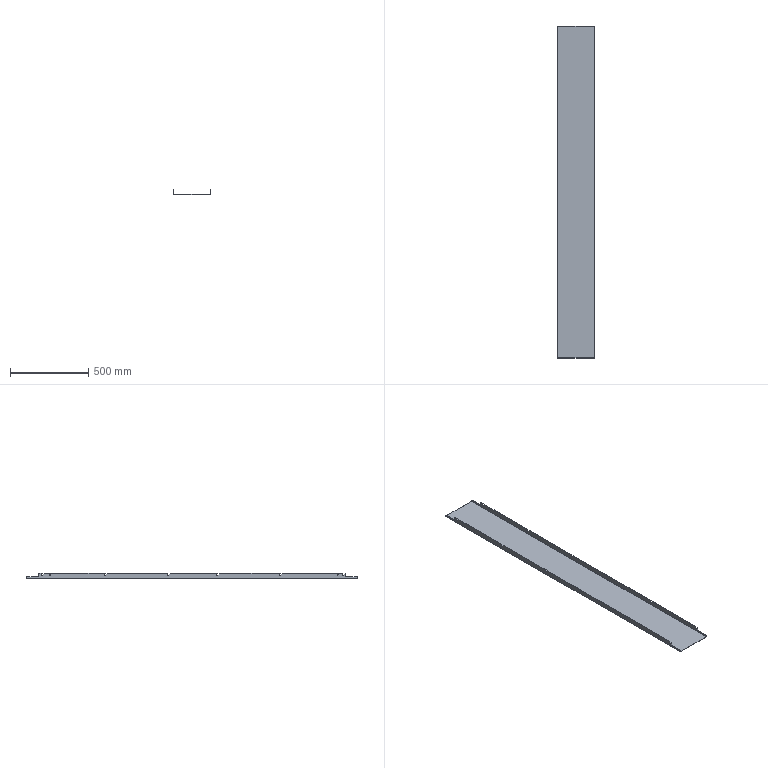Part | SolidWorks | features ICE 4, Chamfer 2, Fillet 1, FlatPattern 1, SMBaseFlange 1, SheetMetal 1 | 1 solid | 102 faces | box 235 x 2116 x 33 mm | volume 746266 mm3 | plane 66 | cylinder 36 | commonest cylinder face diameters 8.2 x24 6 x8 0.4 x2 2.8 x2